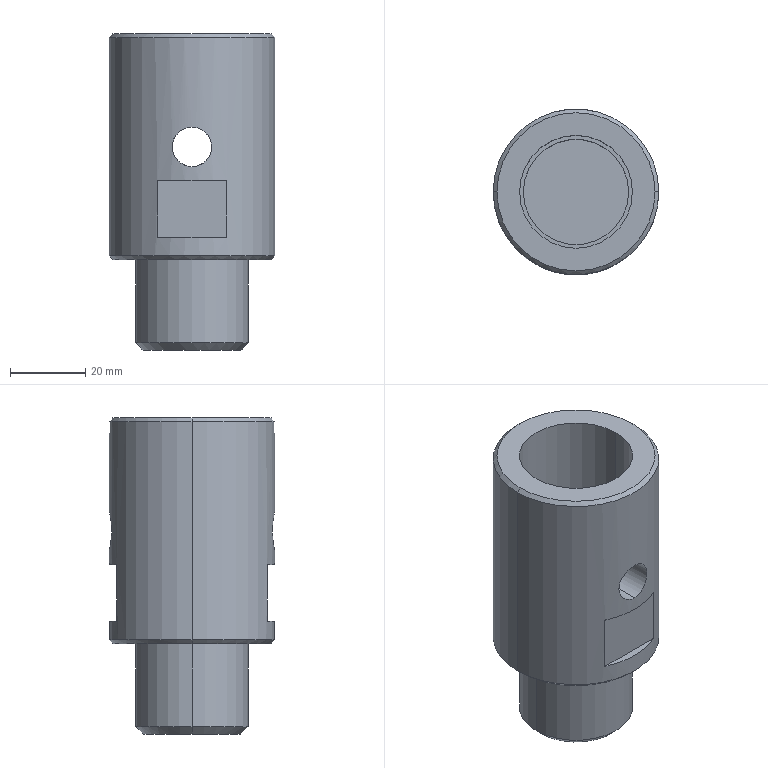Part | STEP file | OP10-108_guide catch | 1 solid | 29 faces | box 44 x 44 x 84 mm | volume 74087 mm3 | cylinder 12 | plane 11 | cone 6 | commonest cylinder face diameters 10.5 x4 30 x4 28 x2 44 x2